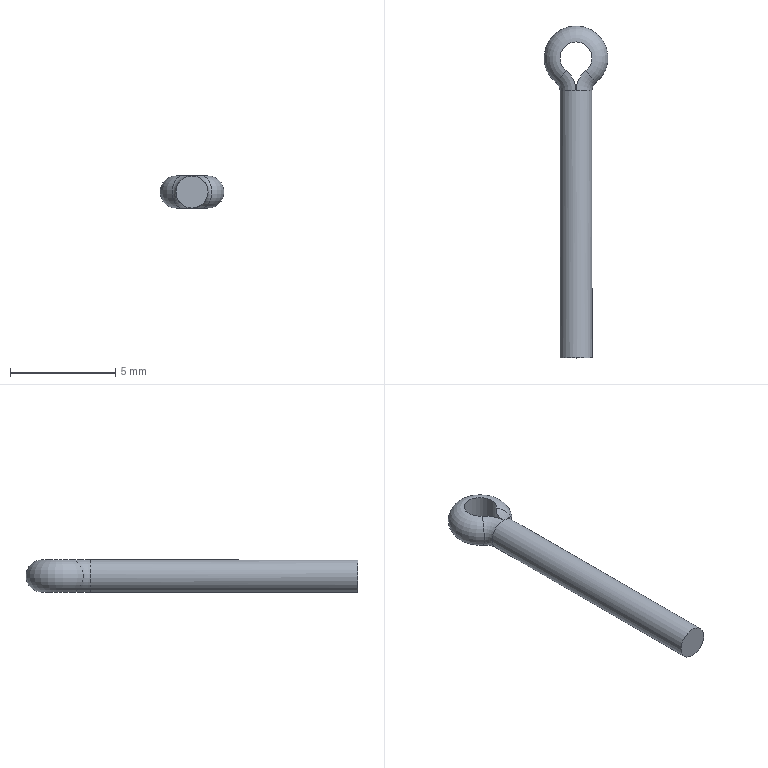Part | NX | features solid 2 | 1 solid | 8 faces | box 3.048 x 15.786 x 1.524 mm | volume 29.558 mm3 | cylinder 4 | torus 3 | plane 1 | commonest cylinder face diameters 1.524 x2 2.438 x2
STEP:
#1=CARTESIAN_POINT('',(-0.4689,13.661,-0.762));
#2=VERTEX_POINT('',#1);
#3=CARTESIAN_POINT('',(-0.4689,13.661,0.762));
#4=VERTEX_POINT('',#3);
#5=CARTESIAN_POINT('',(-0.4689,13.661,-0.762));
#6=DIRECTION('',(0.,0.,1.));
#7=VECTOR('',#6,1000.);
#8=LINE('',#5,#7);
#9=EDGE_CURVE('',#2,#4,#8,.T.);
#10=ORIENTED_EDGE('',*,*,#9,.F.);
#11=CARTESIAN_POINT('',(0.4689,13.661,-0.762));
#12=VERTEX_POINT('',#11);
#13=CARTESIAN_POINT('',(0.,14.262,-0.762));
#14=DIRECTION('',(0.,0.,-1.));
#15=DIRECTION('',(0.,1.,0.));
#16=AXIS2_PLACEMENT_3D('',#13,#14,#15);
#17=CIRCLE('',#16,0.762);
#18=EDGE_CURVE('',#12,#2,#17,.F.);
#19=ORIENTED_EDGE('',*,*,#18,.F.);
#20=CARTESIAN_POINT('',(0.4689,13.661,0.762));
#21=VERTEX_POINT('',#20);
#22=CARTESIAN_POINT('',(0.4689,13.661,-0.762));
#23=DIRECTION('',(0.,0.,1.));
#24=VECTOR('',#23,1000.);
#25=LINE('',#22,#24);
#26=EDGE_CURVE('',#12,#21,#25,.T.);
#27=ORIENTED_EDGE('',*,*,#26,.T.);
#28=CARTESIAN_POINT('',(0.,14.262,0.762));
#29=DIRECTION('',(0.,0.,-1.));
#30=DIRECTION('',(0.,1.,0.));
#31=AXIS2_PLACEMENT_3D('',#28,#29,#30);
#32=CIRCLE('',#31,0.762);
#33=EDGE_CURVE('',#4,#21,#32,.T.);
#34=ORIENTED_EDGE('',*,*,#33,.F.);
#35=EDGE_LOOP('',(#10,#19,#27,#34));
#36=FACE_BOUND('',#35,.T.);
#37=CARTESIAN_POINT('',(0.,14.262,0.));
#38=DIRECTION('',(0.,0.,-1.));
#39=DIRECTION('',(0.,1.,0.));
#40=AXIS2_PLACEMENT_3D('',#37,#38,#39);
#41=CYLINDRICAL_SURFACE('',#40,0.762);
#42=ADVANCED_FACE('',(#36),#41,.F.);
#43=CARTESIAN_POINT('',(-0.4689,13.661,0.));
#44=DIRECTION('',(0.7882,-0.6154,0.));
#45=DIRECTION('',(0.6154,0.7882,0.));
#46=AXIS2_PLACEMENT_3D('',#43,#44,#45);
#47=CIRCLE('',#46,0.762);
#48=EDGE_CURVE('',#4,#2,#47,.T.);
#49=ORIENTED_EDGE('',*,*,#48,.F.);
#50=ORIENTED_EDGE('',*,*,#33,.T.);
#51=CARTESIAN_POINT('',(0.4689,13.661,0.));
#52=DIRECTION('',(0.7882,0.6154,0.));
#53=DIRECTION('',(-0.6154,0.7882,0.));
#54=AXIS2_PLACEMENT_3D('',#51,#52,#53);
#55=CIRCLE('',#54,0.762);
#56=EDGE_CURVE('',#21,#12,#55,.T.);
#57=ORIENTED_EDGE('',*,*,#56,.T.);
#58=ORIENTED_EDGE('',*,*,#18,.T.);
#59=EDGE_LOOP('',(#49,#50,#57,#58));
#60=FACE_BOUND('',#59,.T.);
#61=CARTESIAN_POINT('',(0.,14.262,0.));
#62=DIRECTION('',(0.,0.,-1.));
#63=DIRECTION('',(0.,1.,0.));
#64=AXIS2_PLACEMENT_3D('',#61,#62,#63);
#65=TOROIDAL_SURFACE('',#64,0.762,0.762);
#66=ADVANCED_FACE('',(#60),#65,.T.);
#67=CARTESIAN_POINT('',(0.,12.7,-0.762));
#68=VERTEX_POINT('',#67);
#69=CARTESIAN_POINT('',(0.,12.7,0.762));
#70=VERTEX_POINT('',#69);
#71=CARTESIAN_POINT('',(0.,12.7,-0.762));
#72=DIRECTION('',(0.,0.,1.));
#73=VECTOR('',#72,1000.);
#74=LINE('',#71,#73);
#75=EDGE_CURVE('',#68,#70,#74,.T.);
#76=ORIENTED_EDGE('',*,*,#75,.F.);
#77=CARTESIAN_POINT('',(-1.219,12.7,-0.762));
#78=DIRECTION('',(0.,0.,1.));
#79=DIRECTION('',(0.,-1.,0.));
#80=AXIS2_PLACEMENT_3D('',#77,#78,#79);
#81=CIRCLE('',#80,1.219);
#82=EDGE_CURVE('',#68,#2,#81,.T.);
#83=ORIENTED_EDGE('',*,*,#82,.T.);
#84=ORIENTED_EDGE('',*,*,#9,.T.);
#85=CARTESIAN_POINT('',(-1.219,12.7,0.762));
#86=DIRECTION('',(0.,0.,1.));
#87=DIRECTION('',(0.,-1.,0.));
#88=AXIS2_PLACEMENT_3D('',#85,#86,#87);
#89=CIRCLE('',#88,1.219);
#90=EDGE_CURVE('',#4,#70,#89,.F.);
#91=ORIENTED_EDGE('',*,*,#90,.T.);
#92=EDGE_LOOP('',(#76,#83,#84,#91));
#93=FACE_BOUND('',#92,.T.);
#94=CARTESIAN_POINT('',(-1.219,12.7,0.));
#95=DIRECTION('',(0.,0.,1.));
#96=DIRECTION('',(0.,-1.,0.));
#97=AXIS2_PLACEMENT_3D('',#94,#95,#96);
#98=CYLINDRICAL_SURFACE('',#97,1.219);
#99=ADVANCED_FACE('',(#93),#98,.T.);
#100=CARTESIAN_POINT('',(0.,12.7,0.));
#101=DIRECTION('',(0.,-1.,0.));
#102=DIRECTION('',(1.,0.,0.));
#103=AXIS2_PLACEMENT_3D('',#100,#101,#102);
#104=CIRCLE('',#103,0.762);
#105=EDGE_CURVE('',#70,#68,#104,.T.);
#106=ORIENTED_EDGE('',*,*,#105,.F.);
#107=ORIENTED_EDGE('',*,*,#90,.F.);
#108=ORIENTED_EDGE('',*,*,#48,.T.);
#109=ORIENTED_EDGE('',*,*,#82,.F.);
#110=EDGE_LOOP('',(#106,#107,#108,#109));
#111=FACE_BOUND('',#110,.T.);
#112=CARTESIAN_POINT('',(-1.219,12.7,0.));
#113=DIRECTION('',(0.,0.,1.));
#114=DIRECTION('',(0.,-1.,0.));
#115=AXIS2_PLACEMENT_3D('',#112,#113,#114);
#116=TOROIDAL_SURFACE('',#115,1.219,0.762);
#117=ADVANCED_FACE('',(#111),#116,.T.);
#118=CARTESIAN_POINT('',(0.762,0.,0.));
#119=VERTEX_POINT('',#118);
#120=CARTESIAN_POINT('',(0.,0.,0.));
#121=DIRECTION('',(0.,-1.,0.));
#122=DIRECTION('',(1.,0.,0.));
#123=AXIS2_PLACEMENT_3D('',#120,#121,#122);
#124=CIRCLE('',#123,0.762);
#125=EDGE_CURVE('',#119,#119,#124,.T.);
#126=ORIENTED_EDGE('',*,*,#125,.F.);
#127=EDGE_LOOP('',(#126));
#128=FACE_BOUND('',#127,.T.);
#129=CARTESIAN_POINT('',(0.,12.7,0.));
#130=DIRECTION('',(0.,1.,0.));
#131=DIRECTION('',(-1.,0.,0.));
#132=AXIS2_PLACEMENT_3D('',#129,#130,#131);
#133=CIRCLE('',#132,0.762);
#134=EDGE_CURVE('',#68,#70,#133,.F.);
#135=ORIENTED_EDGE('',*,*,#134,.T.);
#136=ORIENTED_EDGE('',*,*,#105,.T.);
#137=EDGE_LOOP('',(#135,#136));
#138=FACE_BOUND('',#137,.T.);
#139=CARTESIAN_POINT('',(0.,12.7,0.));
#140=DIRECTION('',(0.,-1.,0.));
#141=DIRECTION('',(0.,0.,-1.));
#142=AXIS2_PLACEMENT_3D('',#139,#140,#141);
#143=CYLINDRICAL_SURFACE('',#142,0.762);
#144=ADVANCED_FACE('',(#128,#138),#143,.T.);
#145=ORIENTED_EDGE('',*,*,#125,.T.);
#146=EDGE_LOOP('',(#145));
#147=FACE_BOUND('',#146,.T.);
#148=CARTESIAN_POINT('',(0.,0.,0.));
#149=DIRECTION('',(0.,-1.,0.));
#150=DIRECTION('',(0.,0.,-1.));
#151=AXIS2_PLACEMENT_3D('',#148,#149,#150);
#152=PLANE('',#151);
#153=ADVANCED_FACE('',(#147),#152,.T.);
#154=ORIENTED_EDGE('',*,*,#75,.T.);
#155=CARTESIAN_POINT('',(1.219,12.7,0.762));
#156=DIRECTION('',(0.,0.,-1.));
#157=DIRECTION('',(0.,-1.,0.));
#158=AXIS2_PLACEMENT_3D('',#155,#156,#157);
#159=CIRCLE('',#158,1.219);
#160=EDGE_CURVE('',#21,#70,#159,.F.);
#161=ORIENTED_EDGE('',*,*,#160,.F.);
#162=ORIENTED_EDGE('',*,*,#26,.F.);
#163=CARTESIAN_POINT('',(1.219,12.7,-0.762));
#164=DIRECTION('',(0.,0.,-1.));
#165=DIRECTION('',(0.,-1.,0.));
#166=AXIS2_PLACEMENT_3D('',#163,#164,#165);
#167=CIRCLE('',#166,1.219);
#168=EDGE_CURVE('',#68,#12,#167,.T.);
#169=ORIENTED_EDGE('',*,*,#168,.F.);
#170=EDGE_LOOP('',(#154,#161,#162,#169));
#171=FACE_BOUND('',#170,.T.);
#172=CARTESIAN_POINT('',(1.219,12.7,0.));
#173=DIRECTION('',(0.,0.,1.));
#174=DIRECTION('',(0.,-1.,0.));
#175=AXIS2_PLACEMENT_3D('',#172,#173,#174);
#176=CYLINDRICAL_SURFACE('',#175,1.219);
#177=ADVANCED_FACE('',(#171),#176,.T.);
#178=ORIENTED_EDGE('',*,*,#134,.F.);
#179=ORIENTED_EDGE('',*,*,#168,.T.);
#180=ORIENTED_EDGE('',*,*,#56,.F.);
#181=ORIENTED_EDGE('',*,*,#160,.T.);
#182=EDGE_LOOP('',(#178,#179,#180,#181));
#183=FACE_BOUND('',#182,.T.);
#184=CARTESIAN_POINT('',(1.219,12.7,0.));
#185=DIRECTION('',(0.,0.,1.));
#186=DIRECTION('',(0.,-1.,0.));
#187=AXIS2_PLACEMENT_3D('',#184,#185,#186);
#188=TOROIDAL_SURFACE('',#187,1.219,0.762);
#189=ADVANCED_FACE('',(#183),#188,.T.);
#190=CLOSED_SHELL('',(#42,#66,#99,#117,#144,#153,#177,#189));
#191=MANIFOLD_SOLID_BREP('',#190);
#192=(LENGTH_UNIT()NAMED_UNIT(*)SI_UNIT(.MILLI.,.METRE.));
#193=UNCERTAINTY_MEASURE_WITH_UNIT(LENGTH_MEASURE(0.00001),#192,'','');
#194=(NAMED_UNIT(*)PLANE_ANGLE_UNIT()SI_UNIT($,.RADIAN.));
#195=(NAMED_UNIT(*)SI_UNIT($,.STERADIAN.)SOLID_ANGLE_UNIT());
#196=(GEOMETRIC_REPRESENTATION_CONTEXT(3)GLOBAL_UNCERTAINTY_ASSIGNED_CONTEXT((#193))GLOBAL_UNIT_ASSIGNED_CONTEXT((#192,#194,#195))REPRESENTATION_CONTEXT('',''));
#197=ADVANCED_BREP_SHAPE_REPRESENTATION('',(#191),#196);